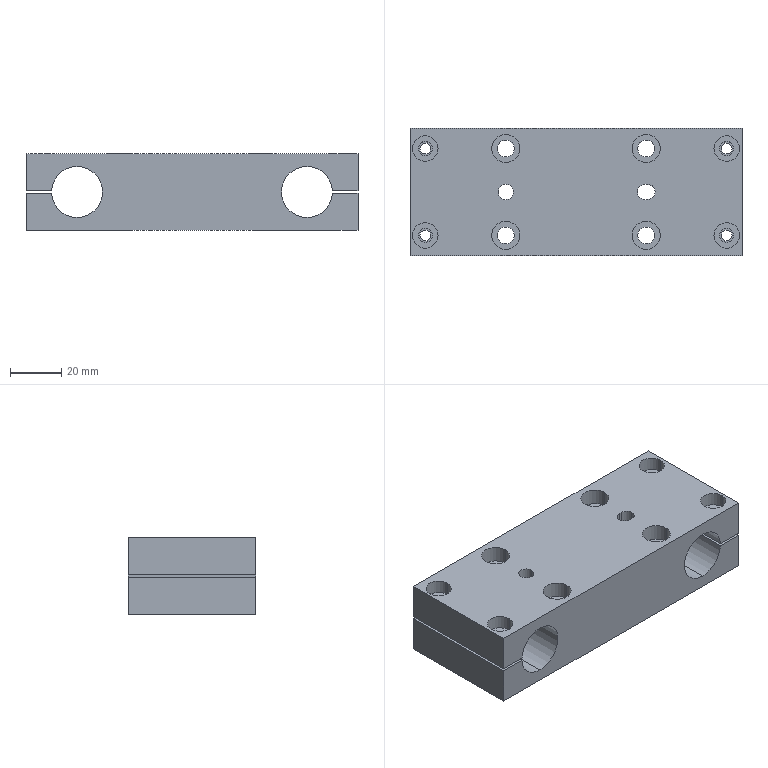Part | STEP file | A11 | 1 solid | 73 faces | box 130 x 50 x 30 mm | volume 151680 mm3 | cylinder 51 | plane 22 | commonest cylinder face diameters 4.2 x8 5.5 x8 6.6 x8 10 x8 11 x8 20 x6